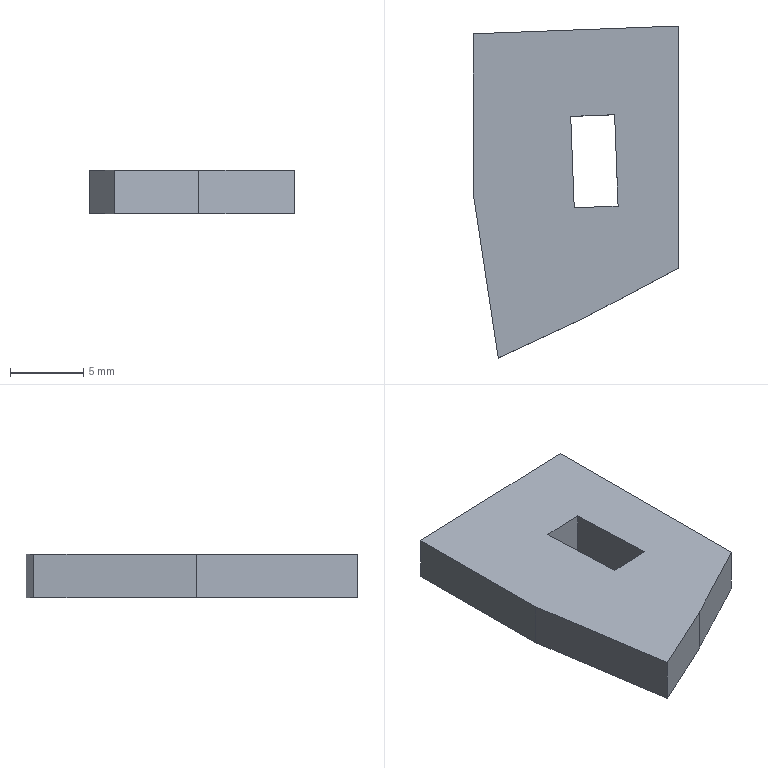Part | SolidWorks | features BaseBody 1 | 1 solid | 12 faces | box 14.02 x 22.667 x 3 mm | volume 747.582 mm3 | plane 7 | spline 5
STEP:
#1=CARTESIAN_POINT('',(-8.823,-6.901,-1.5));
#2=VERTEX_POINT('',#1);
#3=CARTESIAN_POINT('',(-9.061,-0.6622,-1.5));
#4=VERTEX_POINT('',#3);
#5=CARTESIAN_POINT('',(-9.061,-0.6622,-1.5));
#6=DIRECTION('',(-0.03818,0.9993,0.));
#7=VECTOR('',#6,1000.);
#8=LINE('',#5,#7);
#9=EDGE_CURVE('',#2,#4,#8,.T.);
#10=ORIENTED_EDGE('',*,*,#9,.F.);
#11=CARTESIAN_POINT('',(-8.823,-6.901,1.5));
#12=VERTEX_POINT('',#11);
#13=CARTESIAN_POINT('',(-8.823,-6.901,1.5));
#14=DIRECTION('',(0.,0.,-1.));
#15=VECTOR('',#14,1000.);
#16=LINE('',#13,#15);
#17=EDGE_CURVE('',#12,#2,#16,.T.);
#18=ORIENTED_EDGE('',*,*,#17,.F.);
#19=CARTESIAN_POINT('',(-9.061,-0.6622,1.5));
#20=VERTEX_POINT('',#19);
#21=CARTESIAN_POINT('',(-9.061,-0.6622,1.5));
#22=DIRECTION('',(-0.03818,0.9993,0.));
#23=VECTOR('',#22,1000.);
#24=LINE('',#21,#23);
#25=EDGE_CURVE('',#12,#20,#24,.T.);
#26=ORIENTED_EDGE('',*,*,#25,.T.);
#27=CARTESIAN_POINT('',(-9.061,-0.6622,1.5));
#28=DIRECTION('',(0.,0.,-1.));
#29=VECTOR('',#28,1000.);
#30=LINE('',#27,#29);
#31=EDGE_CURVE('',#20,#4,#30,.T.);
#32=ORIENTED_EDGE('',*,*,#31,.T.);
#33=EDGE_LOOP('',(#10,#18,#26,#32));
#34=FACE_OUTER_BOUND('',#33,.T.);
#35=CARTESIAN_POINT('',(-9.061,-0.6622,1.5));
#36=DIRECTION('',(-0.9993,-0.03818,0.));
#37=DIRECTION('',(-0.03818,0.9993,0.));
#38=AXIS2_PLACEMENT_3D('',#35,#36,#37);
#39=PLANE('',#38);
#40=ADVANCED_FACE('',(#34),#39,.T.);
#41=CARTESIAN_POINT('',(-11.82,-7.016,-1.5));
#42=VERTEX_POINT('',#41);
#43=CARTESIAN_POINT('',(-8.823,-6.901,-1.5));
#44=DIRECTION('',(0.9993,0.03818,0.));
#45=VECTOR('',#44,1000.);
#46=LINE('',#43,#45);
#47=EDGE_CURVE('',#42,#2,#46,.T.);
#48=ORIENTED_EDGE('',*,*,#47,.F.);
#49=CARTESIAN_POINT('',(-11.82,-7.016,1.5));
#50=VERTEX_POINT('',#49);
#51=CARTESIAN_POINT('',(-11.82,-7.016,1.5));
#52=DIRECTION('',(0.,0.,-1.));
#53=VECTOR('',#52,1000.);
#54=LINE('',#51,#53);
#55=EDGE_CURVE('',#50,#42,#54,.T.);
#56=ORIENTED_EDGE('',*,*,#55,.F.);
#57=CARTESIAN_POINT('',(-8.823,-6.901,1.5));
#58=DIRECTION('',(0.9993,0.03818,0.));
#59=VECTOR('',#58,1000.);
#60=LINE('',#57,#59);
#61=EDGE_CURVE('',#50,#12,#60,.T.);
#62=ORIENTED_EDGE('',*,*,#61,.T.);
#63=ORIENTED_EDGE('',*,*,#17,.T.);
#64=EDGE_LOOP('',(#48,#56,#62,#63));
#65=FACE_OUTER_BOUND('',#64,.T.);
#66=CARTESIAN_POINT('',(-8.823,-6.901,1.5));
#67=DIRECTION('',(-0.03818,0.9993,0.));
#68=DIRECTION('',(0.,0.,1.));
#69=AXIS2_PLACEMENT_3D('',#66,#67,#68);
#70=PLANE('',#69);
#71=ADVANCED_FACE('',(#65),#70,.T.);
#72=CARTESIAN_POINT('',(-12.059,-0.7768,-1.5));
#73=VERTEX_POINT('',#72);
#74=CARTESIAN_POINT('',(-12.059,-0.7768,-1.5));
#75=DIRECTION('',(0.03818,-0.9993,0.));
#76=VECTOR('',#75,1000.);
#77=LINE('',#74,#76);
#78=EDGE_CURVE('',#73,#42,#77,.T.);
#79=ORIENTED_EDGE('',*,*,#78,.F.);
#80=CARTESIAN_POINT('',(-12.059,-0.7768,1.5));
#81=VERTEX_POINT('',#80);
#82=CARTESIAN_POINT('',(-12.059,-0.7768,1.5));
#83=DIRECTION('',(0.,0.,-1.));
#84=VECTOR('',#83,1000.);
#85=LINE('',#82,#84);
#86=EDGE_CURVE('',#81,#73,#85,.T.);
#87=ORIENTED_EDGE('',*,*,#86,.F.);
#88=CARTESIAN_POINT('',(-12.059,-0.7768,1.5));
#89=DIRECTION('',(0.03818,-0.9993,0.));
#90=VECTOR('',#89,1000.);
#91=LINE('',#88,#90);
#92=EDGE_CURVE('',#81,#50,#91,.T.);
#93=ORIENTED_EDGE('',*,*,#92,.T.);
#94=ORIENTED_EDGE('',*,*,#55,.T.);
#95=EDGE_LOOP('',(#79,#87,#93,#94));
#96=FACE_OUTER_BOUND('',#95,.T.);
#97=CARTESIAN_POINT('',(-12.059,-0.7768,1.5));
#98=DIRECTION('',(0.9993,0.03818,0.));
#99=DIRECTION('',(0.,0.,-1.));
#100=AXIS2_PLACEMENT_3D('',#97,#98,#99);
#101=PLANE('',#100);
#102=ADVANCED_FACE('',(#96),#101,.T.);
#103=CARTESIAN_POINT('',(-9.061,-0.6622,-1.5));
#104=DIRECTION('',(-0.9993,-0.03818,0.));
#105=VECTOR('',#104,1000.);
#106=LINE('',#103,#105);
#107=EDGE_CURVE('',#4,#73,#106,.T.);
#108=ORIENTED_EDGE('',*,*,#107,.F.);
#109=ORIENTED_EDGE('',*,*,#31,.F.);
#110=CARTESIAN_POINT('',(-9.061,-0.6622,1.5));
#111=DIRECTION('',(-0.9993,-0.03818,0.));
#112=VECTOR('',#111,1000.);
#113=LINE('',#110,#112);
#114=EDGE_CURVE('',#20,#81,#113,.T.);
#115=ORIENTED_EDGE('',*,*,#114,.T.);
#116=ORIENTED_EDGE('',*,*,#86,.T.);
#117=EDGE_LOOP('',(#108,#109,#115,#116));
#118=FACE_OUTER_BOUND('',#117,.T.);
#119=CARTESIAN_POINT('',(-9.061,-0.6622,1.5));
#120=DIRECTION('',(0.03818,-0.9993,0.));
#121=DIRECTION('',(0.,0.,-1.));
#122=AXIS2_PLACEMENT_3D('',#119,#120,#121);
#123=PLANE('',#122);
#124=ADVANCED_FACE('',(#118),#123,.T.);
#125=CARTESIAN_POINT('',(-4.688,-11.138,-1.5));
#126=VERTEX_POINT('',#125);
#127=CARTESIAN_POINT('',(-4.688,5.397,-1.5));
#128=VERTEX_POINT('',#127);
#129=CARTESIAN_POINT('',(-4.688,5.397,-1.5));
#130=DIRECTION('',(0.,1.,0.));
#131=VECTOR('',#130,1000.);
#132=LINE('',#129,#131);
#133=EDGE_CURVE('',#126,#128,#132,.T.);
#134=ORIENTED_EDGE('',*,*,#133,.T.);
#135=CARTESIAN_POINT('',(-4.688,5.397,1.5));
#136=VERTEX_POINT('',#135);
#137=CARTESIAN_POINT('',(-4.688,5.397,1.5));
#138=DIRECTION('',(0.,0.,-1.));
#139=VECTOR('',#138,1000.);
#140=LINE('',#137,#139);
#141=EDGE_CURVE('',#136,#128,#140,.T.);
#142=ORIENTED_EDGE('',*,*,#141,.F.);
#143=CARTESIAN_POINT('',(-4.688,-11.138,1.5));
#144=VERTEX_POINT('',#143);
#145=CARTESIAN_POINT('',(-4.688,5.397,1.5));
#146=DIRECTION('',(0.,1.,0.));
#147=VECTOR('',#146,1000.);
#148=LINE('',#145,#147);
#149=EDGE_CURVE('',#144,#136,#148,.T.);
#150=ORIENTED_EDGE('',*,*,#149,.F.);
#151=CARTESIAN_POINT('',(-4.688,-11.138,1.5));
#152=DIRECTION('',(0.,0.,-1.));
#153=VECTOR('',#152,1000.);
#154=LINE('',#151,#153);
#155=EDGE_CURVE('',#144,#126,#154,.T.);
#156=ORIENTED_EDGE('',*,*,#155,.T.);
#157=EDGE_LOOP('',(#134,#142,#150,#156));
#158=FACE_OUTER_BOUND('',#157,.T.);
#159=CARTESIAN_POINT('',(-4.688,5.397,1.5));
#160=DIRECTION('',(-1.,0.,0.));
#161=DIRECTION('',(0.,0.,1.));
#162=AXIS2_PLACEMENT_3D('',#159,#160,#161);
#163=PLANE('',#162);
#164=ADVANCED_FACE('',(#158),#163,.F.);
#165=CARTESIAN_POINT('',(-11.237,-14.597,-1.5));
#166=VERTEX_POINT('',#165);
#167=CARTESIAN_POINT('',(-11.237,-14.597,-1.5));
#168=CARTESIAN_POINT('',(-9.054,-13.443,-1.5));
#169=CARTESIAN_POINT('',(-6.871,-12.291,-1.5));
#170=CARTESIAN_POINT('',(-4.688,-11.138,-1.5));
#171=B_SPLINE_CURVE_WITH_KNOTS('',3,(#167,#168,#169,#170),.UNSPECIFIED.,.F.,.F.,(4,4),(0.7273,0.8182),.UNSPECIFIED.);
#172=EDGE_CURVE('',#166,#126,#171,.T.);
#173=ORIENTED_EDGE('',*,*,#172,.T.);
#174=ORIENTED_EDGE('',*,*,#155,.F.);
#175=CARTESIAN_POINT('',(-11.237,-14.597,1.5));
#176=VERTEX_POINT('',#175);
#177=CARTESIAN_POINT('',(-11.237,-14.597,1.5));
#178=CARTESIAN_POINT('',(-9.054,-13.443,1.5));
#179=CARTESIAN_POINT('',(-6.871,-12.291,1.5));
#180=CARTESIAN_POINT('',(-4.688,-11.138,1.5));
#181=B_SPLINE_CURVE_WITH_KNOTS('',3,(#177,#178,#179,#180),.UNSPECIFIED.,.F.,.F.,(4,4),(0.7273,0.8182),.UNSPECIFIED.);
#182=EDGE_CURVE('',#176,#144,#181,.T.);
#183=ORIENTED_EDGE('',*,*,#182,.F.);
#184=CARTESIAN_POINT('',(-11.237,-14.597,1.5));
#185=DIRECTION('',(0.,0.,-1.));
#186=VECTOR('',#185,1000.);
#187=LINE('',#184,#186);
#188=EDGE_CURVE('',#176,#166,#187,.T.);
#189=ORIENTED_EDGE('',*,*,#188,.T.);
#190=EDGE_LOOP('',(#173,#174,#183,#189));
#191=FACE_OUTER_BOUND('',#190,.T.);
#192=CARTESIAN_POINT('',(-11.237,-14.597,1.5));
#193=CARTESIAN_POINT('',(-11.237,-14.597,-1.5));
#194=CARTESIAN_POINT('',(-9.054,-13.443,1.5));
#195=CARTESIAN_POINT('',(-9.054,-13.443,-1.5));
#196=CARTESIAN_POINT('',(-6.871,-12.291,1.5));
#197=CARTESIAN_POINT('',(-6.871,-12.291,-1.5));
#198=CARTESIAN_POINT('',(-4.688,-11.138,1.5));
#199=CARTESIAN_POINT('',(-4.688,-11.138,-1.5));
#200=B_SPLINE_SURFACE_WITH_KNOTS('',3,1,((#192,#193),(#194,#195),(#196,#197),(#198,#199)),.UNSPECIFIED.,.F.,.F.,.F.,(4,4),(2,2),(0.7273,0.8182),(0.,1.),.UNSPECIFIED.);
#201=ADVANCED_FACE('',(#191),#200,.F.);
#202=CARTESIAN_POINT('',(-17.014,-17.271,-1.5));
#203=VERTEX_POINT('',#202);
#204=CARTESIAN_POINT('',(-17.014,-17.271,-1.5));
#205=CARTESIAN_POINT('',(-15.089,-16.38,-1.5));
#206=CARTESIAN_POINT('',(-13.164,-15.49,-1.5));
#207=CARTESIAN_POINT('',(-11.237,-14.597,-1.5));
#208=B_SPLINE_CURVE_WITH_KNOTS('',3,(#204,#205,#206,#207),.UNSPECIFIED.,.F.,.F.,(4,4),(0.6364,0.7273),.UNSPECIFIED.);
#209=EDGE_CURVE('',#203,#166,#208,.T.);
#210=ORIENTED_EDGE('',*,*,#209,.T.);
#211=ORIENTED_EDGE('',*,*,#188,.F.);
#212=CARTESIAN_POINT('',(-17.014,-17.271,1.5));
#213=VERTEX_POINT('',#212);
#214=CARTESIAN_POINT('',(-17.014,-17.271,1.5));
#215=CARTESIAN_POINT('',(-15.089,-16.38,1.5));
#216=CARTESIAN_POINT('',(-13.164,-15.49,1.5));
#217=CARTESIAN_POINT('',(-11.237,-14.597,1.5));
#218=B_SPLINE_CURVE_WITH_KNOTS('',3,(#214,#215,#216,#217),.UNSPECIFIED.,.F.,.F.,(4,4),(0.6364,0.7273),.UNSPECIFIED.);
#219=EDGE_CURVE('',#213,#176,#218,.T.);
#220=ORIENTED_EDGE('',*,*,#219,.F.);
#221=CARTESIAN_POINT('',(-17.014,-17.271,1.5));
#222=DIRECTION('',(0.,0.,-1.));
#223=VECTOR('',#222,1000.);
#224=LINE('',#221,#223);
#225=EDGE_CURVE('',#213,#203,#224,.T.);
#226=ORIENTED_EDGE('',*,*,#225,.T.);
#227=EDGE_LOOP('',(#210,#211,#220,#226));
#228=FACE_OUTER_BOUND('',#227,.T.);
#229=CARTESIAN_POINT('',(-17.014,-17.271,1.5));
#230=CARTESIAN_POINT('',(-17.014,-17.271,-1.5));
#231=CARTESIAN_POINT('',(-15.089,-16.38,1.5));
#232=CARTESIAN_POINT('',(-15.089,-16.38,-1.5));
#233=CARTESIAN_POINT('',(-13.164,-15.49,1.5));
#234=CARTESIAN_POINT('',(-13.164,-15.49,-1.5));
#235=CARTESIAN_POINT('',(-11.237,-14.597,1.5));
#236=CARTESIAN_POINT('',(-11.237,-14.597,-1.5));
#237=B_SPLINE_SURFACE_WITH_KNOTS('',3,1,((#229,#230),(#231,#232),(#233,#234),(#235,#236)),.UNSPECIFIED.,.F.,.F.,.F.,(4,4),(2,2),(0.6364,0.7273),(0.,1.),.UNSPECIFIED.);
#238=ADVANCED_FACE('',(#228),#237,.F.);
#239=CARTESIAN_POINT('',(-18.686,-6.257,-1.5));
#240=VERTEX_POINT('',#239);
#241=CARTESIAN_POINT('',(-18.686,-6.257,-1.5));
#242=CARTESIAN_POINT('',(-18.129,-9.928,-1.5));
#243=CARTESIAN_POINT('',(-17.572,-13.598,-1.5));
#244=CARTESIAN_POINT('',(-17.014,-17.271,-1.5));
#245=B_SPLINE_CURVE_WITH_KNOTS('',3,(#241,#242,#243,#244),.UNSPECIFIED.,.F.,.F.,(4,4),(0.5455,0.6364),.UNSPECIFIED.);
#246=EDGE_CURVE('',#240,#203,#245,.T.);
#247=ORIENTED_EDGE('',*,*,#246,.T.);
#248=ORIENTED_EDGE('',*,*,#225,.F.);
#249=CARTESIAN_POINT('',(-18.686,-6.257,1.5));
#250=VERTEX_POINT('',#249);
#251=CARTESIAN_POINT('',(-18.686,-6.257,1.5));
#252=CARTESIAN_POINT('',(-18.129,-9.928,1.5));
#253=CARTESIAN_POINT('',(-17.572,-13.598,1.5));
#254=CARTESIAN_POINT('',(-17.014,-17.271,1.5));
#255=B_SPLINE_CURVE_WITH_KNOTS('',3,(#251,#252,#253,#254),.UNSPECIFIED.,.F.,.F.,(4,4),(0.5455,0.6364),.UNSPECIFIED.);
#256=EDGE_CURVE('',#250,#213,#255,.T.);
#257=ORIENTED_EDGE('',*,*,#256,.F.);
#258=CARTESIAN_POINT('',(-18.686,-6.257,1.5));
#259=DIRECTION('',(0.,0.,-1.));
#260=VECTOR('',#259,1000.);
#261=LINE('',#258,#260);
#262=EDGE_CURVE('',#250,#240,#261,.T.);
#263=ORIENTED_EDGE('',*,*,#262,.T.);
#264=EDGE_LOOP('',(#247,#248,#257,#263));
#265=FACE_OUTER_BOUND('',#264,.T.);
#266=CARTESIAN_POINT('',(-18.686,-6.257,1.5));
#267=CARTESIAN_POINT('',(-18.686,-6.257,-1.5));
#268=CARTESIAN_POINT('',(-18.129,-9.928,1.5));
#269=CARTESIAN_POINT('',(-18.129,-9.928,-1.5));
#270=CARTESIAN_POINT('',(-17.572,-13.598,1.5));
#271=CARTESIAN_POINT('',(-17.572,-13.598,-1.5));
#272=CARTESIAN_POINT('',(-17.014,-17.271,1.5));
#273=CARTESIAN_POINT('',(-17.014,-17.271,-1.5));
#274=B_SPLINE_SURFACE_WITH_KNOTS('',3,1,((#266,#267),(#268,#269),(#270,#271),(#272,#273)),.UNSPECIFIED.,.F.,.F.,.F.,(4,4),(2,2),(0.5455,0.6364),(0.,1.),.UNSPECIFIED.);
#275=ADVANCED_FACE('',(#265),#274,.F.);
#276=CARTESIAN_POINT('',(-18.708,4.865,-1.5));
#277=VERTEX_POINT('',#276);
#278=CARTESIAN_POINT('',(-18.708,4.865,-1.5));
#279=CARTESIAN_POINT('',(-18.7,1.157,-1.5));
#280=CARTESIAN_POINT('',(-18.692,-2.549,-1.5));
#281=CARTESIAN_POINT('',(-18.686,-6.257,-1.5));
#282=B_SPLINE_CURVE_WITH_KNOTS('',3,(#278,#279,#280,#281),.UNSPECIFIED.,.F.,.F.,(4,4),(0.4545,0.5455),.UNSPECIFIED.);
#283=EDGE_CURVE('',#277,#240,#282,.T.);
#284=ORIENTED_EDGE('',*,*,#283,.T.);
#285=ORIENTED_EDGE('',*,*,#262,.F.);
#286=CARTESIAN_POINT('',(-18.708,4.865,1.5));
#287=VERTEX_POINT('',#286);
#288=CARTESIAN_POINT('',(-18.708,4.865,1.5));
#289=CARTESIAN_POINT('',(-18.7,1.157,1.5));
#290=CARTESIAN_POINT('',(-18.692,-2.549,1.5));
#291=CARTESIAN_POINT('',(-18.686,-6.257,1.5));
#292=B_SPLINE_CURVE_WITH_KNOTS('',3,(#288,#289,#290,#291),.UNSPECIFIED.,.F.,.F.,(4,4),(0.4545,0.5455),.UNSPECIFIED.);
#293=EDGE_CURVE('',#287,#250,#292,.T.);
#294=ORIENTED_EDGE('',*,*,#293,.F.);
#295=CARTESIAN_POINT('',(-18.708,4.865,1.5));
#296=DIRECTION('',(0.,0.,-1.));
#297=VECTOR('',#296,1000.);
#298=LINE('',#295,#297);
#299=EDGE_CURVE('',#287,#277,#298,.T.);
#300=ORIENTED_EDGE('',*,*,#299,.T.);
#301=EDGE_LOOP('',(#284,#285,#294,#300));
#302=FACE_OUTER_BOUND('',#301,.T.);
#303=CARTESIAN_POINT('',(-18.708,4.865,1.5));
#304=CARTESIAN_POINT('',(-18.708,4.865,-1.5));
#305=CARTESIAN_POINT('',(-18.7,1.157,1.5));
#306=CARTESIAN_POINT('',(-18.7,1.157,-1.5));
#307=CARTESIAN_POINT('',(-18.692,-2.549,1.5));
#308=CARTESIAN_POINT('',(-18.692,-2.549,-1.5));
#309=CARTESIAN_POINT('',(-18.686,-6.257,1.5));
#310=CARTESIAN_POINT('',(-18.686,-6.257,-1.5));
#311=B_SPLINE_SURFACE_WITH_KNOTS('',3,1,((#303,#304),(#305,#306),(#307,#308),(#309,#310)),.UNSPECIFIED.,.F.,.F.,.F.,(4,4),(2,2),(0.4545,0.5455),(0.,1.),.UNSPECIFIED.);
#312=ADVANCED_FACE('',(#302),#311,.F.);
#313=CARTESIAN_POINT('',(-4.688,5.397,-1.5));
#314=CARTESIAN_POINT('',(-9.363,5.218,-1.5));
#315=CARTESIAN_POINT('',(-14.035,5.041,-1.5));
#316=CARTESIAN_POINT('',(-18.708,4.865,-1.5));
#317=B_SPLINE_CURVE_WITH_KNOTS('',3,(#313,#314,#315,#316),.UNSPECIFIED.,.F.,.F.,(4,4),(0.3636,0.4545),.UNSPECIFIED.);
#318=EDGE_CURVE('',#128,#277,#317,.T.);
#319=ORIENTED_EDGE('',*,*,#318,.T.);
#320=ORIENTED_EDGE('',*,*,#299,.F.);
#321=CARTESIAN_POINT('',(-4.688,5.397,1.5));
#322=CARTESIAN_POINT('',(-9.363,5.218,1.5));
#323=CARTESIAN_POINT('',(-14.035,5.041,1.5));
#324=CARTESIAN_POINT('',(-18.708,4.865,1.5));
#325=B_SPLINE_CURVE_WITH_KNOTS('',3,(#321,#322,#323,#324),.UNSPECIFIED.,.F.,.F.,(4,4),(0.3636,0.4545),.UNSPECIFIED.);
#326=EDGE_CURVE('',#136,#287,#325,.T.);
#327=ORIENTED_EDGE('',*,*,#326,.F.);
#328=ORIENTED_EDGE('',*,*,#141,.T.);
#329=EDGE_LOOP('',(#319,#320,#327,#328));
#330=FACE_OUTER_BOUND('',#329,.T.);
#331=CARTESIAN_POINT('',(-4.688,5.397,1.5));
#332=CARTESIAN_POINT('',(-4.688,5.397,-1.5));
#333=CARTESIAN_POINT('',(-9.363,5.218,1.5));
#334=CARTESIAN_POINT('',(-9.363,5.218,-1.5));
#335=CARTESIAN_POINT('',(-14.035,5.041,1.5));
#336=CARTESIAN_POINT('',(-14.035,5.041,-1.5));
#337=CARTESIAN_POINT('',(-18.708,4.865,1.5));
#338=CARTESIAN_POINT('',(-18.708,4.865,-1.5));
#339=B_SPLINE_SURFACE_WITH_KNOTS('',3,1,((#331,#332),(#333,#334),(#335,#336),(#337,#338)),.UNSPECIFIED.,.F.,.F.,.F.,(4,4),(2,2),(0.3636,0.4545),(0.,1.),.UNSPECIFIED.);
#340=ADVANCED_FACE('',(#330),#339,.F.);
#341=ORIENTED_EDGE('',*,*,#107,.T.);
#342=ORIENTED_EDGE('',*,*,#78,.T.);
#343=ORIENTED_EDGE('',*,*,#47,.T.);
#344=ORIENTED_EDGE('',*,*,#9,.T.);
#345=EDGE_LOOP('',(#341,#342,#343,#344));
#346=FACE_BOUND('',#345,.T.);
#347=ORIENTED_EDGE('',*,*,#318,.F.);
#348=ORIENTED_EDGE('',*,*,#133,.F.);
#349=ORIENTED_EDGE('',*,*,#172,.F.);
#350=ORIENTED_EDGE('',*,*,#209,.F.);
#351=ORIENTED_EDGE('',*,*,#246,.F.);
#352=ORIENTED_EDGE('',*,*,#283,.F.);
#353=EDGE_LOOP('',(#347,#348,#349,#350,#351,#352));
#354=FACE_OUTER_BOUND('',#353,.T.);
#355=CARTESIAN_POINT('',(-11.699,5.13,-1.5));
#356=DIRECTION('',(0.,0.,1.));
#357=DIRECTION('',(1.,0.,0.));
#358=AXIS2_PLACEMENT_3D('',#355,#356,#357);
#359=PLANE('',#358);
#360=ADVANCED_FACE('',(#346,#354),#359,.F.);
#361=ORIENTED_EDGE('',*,*,#92,.F.);
#362=ORIENTED_EDGE('',*,*,#114,.F.);
#363=ORIENTED_EDGE('',*,*,#25,.F.);
#364=ORIENTED_EDGE('',*,*,#61,.F.);
#365=EDGE_LOOP('',(#361,#362,#363,#364));
#366=FACE_BOUND('',#365,.T.);
#367=ORIENTED_EDGE('',*,*,#326,.T.);
#368=ORIENTED_EDGE('',*,*,#293,.T.);
#369=ORIENTED_EDGE('',*,*,#256,.T.);
#370=ORIENTED_EDGE('',*,*,#219,.T.);
#371=ORIENTED_EDGE('',*,*,#182,.T.);
#372=ORIENTED_EDGE('',*,*,#149,.T.);
#373=EDGE_LOOP('',(#367,#368,#369,#370,#371,#372));
#374=FACE_OUTER_BOUND('',#373,.T.);
#375=CARTESIAN_POINT('',(-11.699,5.13,1.5));
#376=DIRECTION('',(0.,0.,1.));
#377=DIRECTION('',(1.,0.,0.));
#378=AXIS2_PLACEMENT_3D('',#375,#376,#377);
#379=PLANE('',#378);
#380=ADVANCED_FACE('',(#366,#374),#379,.T.);
#381=CLOSED_SHELL('',(#40,#71,#102,#124,#164,#201,#238,#275,#312,#340,#360,#380));
#382=MANIFOLD_SOLID_BREP('',#381);
#383=CARTESIAN_POINT('',(0.,0.,0.));
#384=DIRECTION('',(0.,0.,1.));
#385=DIRECTION('',(1.,0.,0.));
#386=AXIS2_PLACEMENT_3D('',#383,#384,#385);
#387=(LENGTH_UNIT()NAMED_UNIT(*)SI_UNIT(.MILLI.,.METRE.));
#388=UNCERTAINTY_MEASURE_WITH_UNIT(LENGTH_MEASURE(0.00001),#387,'','');
#389=(NAMED_UNIT(*)PLANE_ANGLE_UNIT()SI_UNIT($,.RADIAN.));
#390=(NAMED_UNIT(*)SI_UNIT($,.STERADIAN.)SOLID_ANGLE_UNIT());
#391=(GEOMETRIC_REPRESENTATION_CONTEXT(3)GLOBAL_UNCERTAINTY_ASSIGNED_CONTEXT((#388))GLOBAL_UNIT_ASSIGNED_CONTEXT((#387,#389,#390))REPRESENTATION_CONTEXT('',''));
#392=ADVANCED_BREP_SHAPE_REPRESENTATION('',(#382,#386),#391);